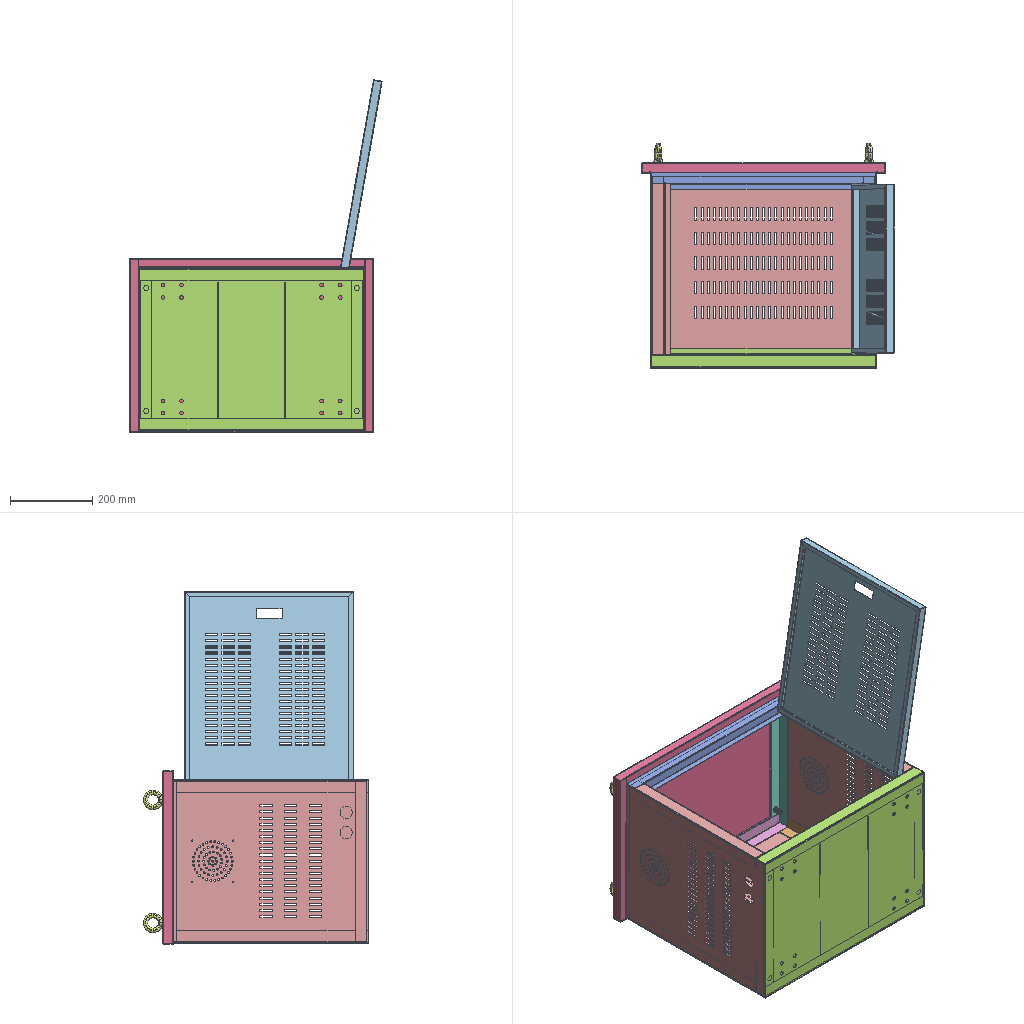Assembly | SolidWorks | 12 different items | 24 placed | box 615 x 549 x 859 mm
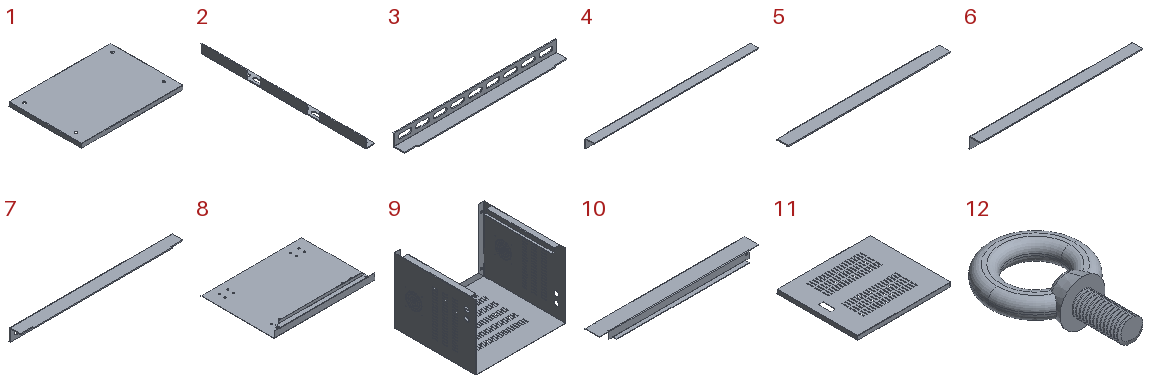Parts list (item | quantity | size | volume | features):
1 | x1 | 593 x 423 x 25 mm | 482972 mm3 | features EdgeFlange 3, CornerFeat 1, Cut 1, FlatPattern 1, SMBaseFlange 1, SheetMetal 1
2 | x1 | 30 x 530 x 30 mm | 60196 mm3 | features ICE 2, EdgeFlange 1, FlatPattern 1, LPattern 1, SMBaseFlange 1, SheetMetal 1
3 | x1 | 390 x 30 x 30 mm | 47297 mm3 | features MirrorStock 1
4 | x4 | 546 x 30 x 30 mm | 77462 mm3 | features EdgeFlange 1, FlatPattern 1, SMBaseFlange 1, SheetMetal 1
5 | x4 | 391 x 30 x 30 mm | 50792 mm3 | features SMBaseFlange 2, Cut 1, EdgeFlange 1, FlatPattern 1, SheetMetal 1
6 | x4 | 435.5 x 30 x 30 mm | 61785 mm3 | features EdgeFlange 1, FlatPattern 1, SMBaseFlange 1, SheetMetal 1
7 | x1 | 390 x 30 x 30 mm | 47297 mm3 | features ICE 2, EdgeFlange 1, FlatPattern 1, SMBaseFlange 1, SheetMetal 1
8 | x1 | 547 x 398.5 x 48.5 mm | 377197 mm3 | features EdgeFlange 3, ICE 2, MirrorPattern 2, FlatPattern 1, SMBaseFlange 1, SheetMetal 1
9 | x1 | 550 x 500 x 400 mm | 1097437 mm3 | features ICE 6, EdgeFlange 5, LPattern 3, FlatPattern 1, SMBaseFlange 1, SheetMetal 1
10 | x1 | 547 x 63.5 x 30 mm | 85940 mm3 | features EdgeFlange 3, FlatPattern 1, ICE 1, SMBaseFlange 1, SheetMetal 1
11 | x1 | 476 x 412.001 x 21.5 mm | 343155 mm3 | features ICE 3, LPattern 3, EdgeFlange 2, CornerFeat 1, FlatPattern 1, SMBaseFlange 1, SheetMetal 1
12 | x4 | 48 x 73 x 23 mm | 14602 mm3 | features Boss 2, Fillet 2, Extrusion 1, Helix 1, SweepCut 1
Mates (type | each side: item.copy, entity, surface, feature):
Coincident | 9.1 face plane Edge-Flange2 | 10.1 face plane Base-Flange1
Coincident | 9.1 face plane Edge-Flange5 | 10.1 face plane Base-Flange1
Coincident | 9.1 face plane Edge-Flange1 | 10.1 face plane Base-Flange1
Coincident | 9.1 face plane Edge-Flange5 | 10.1 face plane Edge-Flange3
Coincident | 9.1 face plane Edge-Flange2 | 8.1 face plane Edge-Flange1
Coincident | 9.1 face plane Edge-Flange1 | 8.1 face plane Edge-Flange1
Coincident | 9.1 face plane Edge-Flange1 | 8.1 face plane Base-Flange1
Coincident | 9.1 face plane Edge-Flange5 | 4.1 face plane Edge-Flange1
Coincident | 9.1 face plane Base-Flange1 | 4.1 face plane Base-Flange1
Coincident | 9.1 face plane Edge-Flange1 | 4.1 face plane Edge-Flange1
Coincident | 10.1 face plane Edge-Flange3 | 4.2 face plane Edge-Flange1
Coincident | 9.1 face plane Edge-Flange1 | 4.2 face plane Edge-Flange1
Coincident | 10.1 face plane Base-Flange1 | 4.2 face plane Base-Flange1
Coincident | 9.1 face plane Edge-Flange1 | 5.1 face plane Base-Flange1
Coincident | 9.1 face plane Edge-Flange5 | 5.1 face plane Edge-Flange1
Coincident | 4.1 face plane Edge-Flange1 | 5.1 face plane Edge-Flange1
Coincident | 9.1 face plane Edge-Flange1 | 6.1 face plane Edge-Flange1
Coincident | 9.1 face plane Base-Flange1 | 6.1 face plane Base-Flange1
Coincident | 4.1 face plane Base-Flange1 | 6.1 face plane Base-Flange1
Coincident | 8.1 face plane Base-Flange1 | 7.1 face plane Base-Flange1
Coincident | 4.3 face plane Base-Flange1 | 7.1 face plane Edge-Flange1
DistanceDim | 3.1 face plane TA0715-Rib4 Mirror | 7.1 face plane Base-Flange1
Coincident | 9.1 face plane Edge-Flange5 | 1.1 face plane Base-Flange1
DistanceDim | 1.1 face plane Edge-Flange2 | 9.1 face plane Edge-Flange1
Coincident | 9.1 face plane Base-Flange1 | 1.1 face plane Edge-Flange1
DistanceDim | 11.1 face plane Edge-Flange1 | 10.1 face plane Edge-Flange1
Concentric | 10.1 face cylinder Cut-Extrude1 | 11.1 face cylinder Cut-Extrude1
LimitPlanarAngleDim | 11.1 face plane Base-Flange1 | 9.1 face plane Edge-Flange2
Concentric | 1.1 edge | 12.1 edge
Coincident | 1.1 face plane Base-Flange1 | 12.1 face plane Boss-Extrude1
Coincident | 3.1 face plane TA0715-Rib4 Mirror | 2.1 face plane Base-Flange1